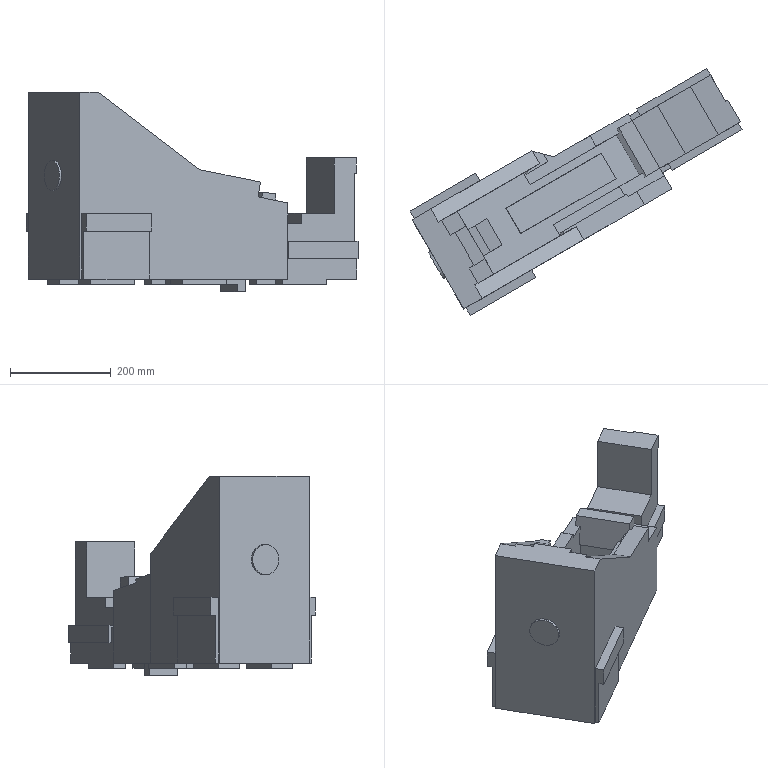Part | NX | features solid 2 | 1 solid | 155 faces | box 657.667 x 489.112 x 394.943 mm | volume 20714629 mm3 | plane 154 | cylinder 1 | commonest cylinder face diameters 60 x1